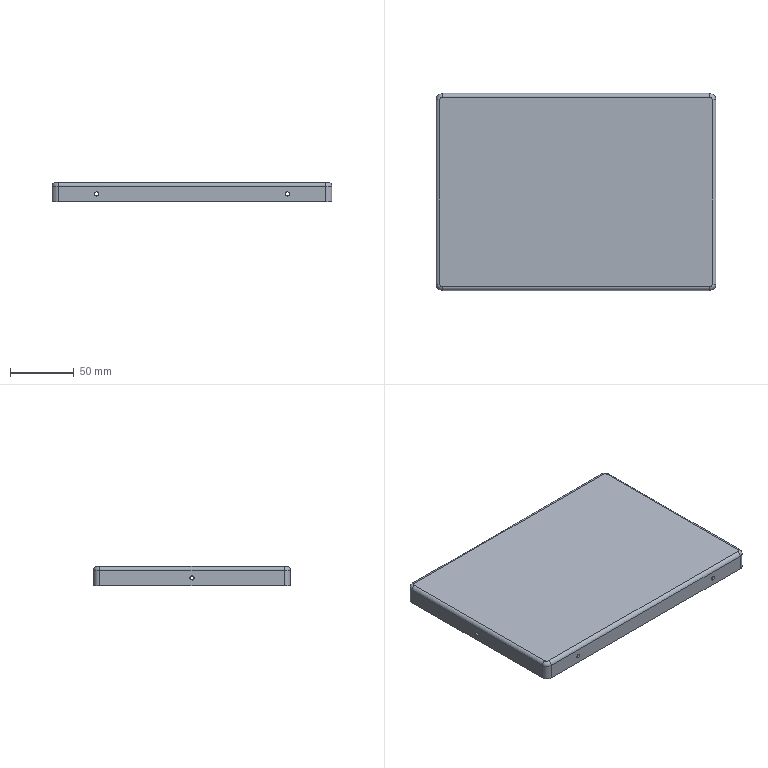Part | NX | features BREP 1 | 1 solid | 47 faces | box 220 x 155 x 15 mm | volume 85900 mm3 | cylinder 28 | plane 11 | torus 8 | commonest cylinder face diameters 3.3 x12 6 x8 2 x4 10 x4
STEP:
#1=CARTESIAN_POINT('',(108.,0.,7.65));
#2=VERTEX_POINT('',#1);
#3=CARTESIAN_POINT('',(110.,0.,7.65));
#4=VERTEX_POINT('',#3);
#5=CARTESIAN_POINT('',(110.,0.,7.65));
#6=DIRECTION('',(1.,0.,0.));
#7=VECTOR('',#6,1000.);
#8=LINE('',#5,#7);
#9=EDGE_CURVE('',#2,#4,#8,.T.);
#10=ORIENTED_EDGE('',*,*,#9,.F.);
#11=CARTESIAN_POINT('',(108.,0.,4.35));
#12=VERTEX_POINT('',#11);
#13=CARTESIAN_POINT('',(108.,0.,6.));
#14=DIRECTION('',(-1.,0.,0.));
#15=DIRECTION('',(0.,0.,1.));
#16=AXIS2_PLACEMENT_3D('',#13,#14,#15);
#17=CIRCLE('',#16,1.65);
#18=EDGE_CURVE('',#2,#12,#17,.T.);
#19=ORIENTED_EDGE('',*,*,#18,.T.);
#20=CARTESIAN_POINT('',(110.,0.,4.35));
#21=VERTEX_POINT('',#20);
#22=CARTESIAN_POINT('',(110.,0.,4.35));
#23=DIRECTION('',(1.,0.,0.));
#24=VECTOR('',#23,1000.);
#25=LINE('',#22,#24);
#26=EDGE_CURVE('',#12,#21,#25,.T.);
#27=ORIENTED_EDGE('',*,*,#26,.T.);
#28=CARTESIAN_POINT('',(110.,0.,6.));
#29=DIRECTION('',(1.,0.,0.));
#30=DIRECTION('',(0.,0.,-1.));
#31=AXIS2_PLACEMENT_3D('',#28,#29,#30);
#32=CIRCLE('',#31,1.65);
#33=EDGE_CURVE('',#21,#4,#32,.T.);
#34=ORIENTED_EDGE('',*,*,#33,.T.);
#35=EDGE_LOOP('',(#10,#19,#27,#34));
#36=FACE_BOUND('',#35,.T.);
#37=CARTESIAN_POINT('',(110.,0.,6.));
#38=DIRECTION('',(1.,0.,0.));
#39=DIRECTION('',(0.,0.,-1.));
#40=AXIS2_PLACEMENT_3D('',#37,#38,#39);
#41=CYLINDRICAL_SURFACE('',#40,1.65);
#42=ADVANCED_FACE('',(#36),#41,.F.);
#43=CARTESIAN_POINT('',(-110.,0.,7.65));
#44=VERTEX_POINT('',#43);
#45=CARTESIAN_POINT('',(-108.,0.,7.65));
#46=VERTEX_POINT('',#45);
#47=CARTESIAN_POINT('',(110.,0.,7.65));
#48=DIRECTION('',(1.,0.,0.));
#49=VECTOR('',#48,1000.);
#50=LINE('',#47,#49);
#51=EDGE_CURVE('',#44,#46,#50,.T.);
#52=ORIENTED_EDGE('',*,*,#51,.F.);
#53=CARTESIAN_POINT('',(-110.,0.,4.35));
#54=VERTEX_POINT('',#53);
#55=CARTESIAN_POINT('',(-110.,0.,6.));
#56=DIRECTION('',(1.,0.,0.));
#57=DIRECTION('',(0.,0.,-1.));
#58=AXIS2_PLACEMENT_3D('',#55,#56,#57);
#59=CIRCLE('',#58,1.65);
#60=EDGE_CURVE('',#54,#44,#59,.T.);
#61=ORIENTED_EDGE('',*,*,#60,.F.);
#62=CARTESIAN_POINT('',(-108.,0.,4.35));
#63=VERTEX_POINT('',#62);
#64=CARTESIAN_POINT('',(110.,0.,4.35));
#65=DIRECTION('',(1.,0.,0.));
#66=VECTOR('',#65,1000.);
#67=LINE('',#64,#66);
#68=EDGE_CURVE('',#54,#63,#67,.T.);
#69=ORIENTED_EDGE('',*,*,#68,.T.);
#70=CARTESIAN_POINT('',(-108.,0.,6.));
#71=DIRECTION('',(1.,0.,0.));
#72=DIRECTION('',(0.,0.,-1.));
#73=AXIS2_PLACEMENT_3D('',#70,#71,#72);
#74=CIRCLE('',#73,1.65);
#75=EDGE_CURVE('',#63,#46,#74,.T.);
#76=ORIENTED_EDGE('',*,*,#75,.T.);
#77=EDGE_LOOP('',(#52,#61,#69,#76));
#78=FACE_BOUND('',#77,.T.);
#79=CARTESIAN_POINT('',(110.,0.,6.));
#80=DIRECTION('',(1.,0.,0.));
#81=DIRECTION('',(0.,0.,-1.));
#82=AXIS2_PLACEMENT_3D('',#79,#80,#81);
#83=CYLINDRICAL_SURFACE('',#82,1.65);
#84=ADVANCED_FACE('',(#78),#83,.F.);
#85=CARTESIAN_POINT('',(-75.,77.5,7.65));
#86=VERTEX_POINT('',#85);
#87=CARTESIAN_POINT('',(-75.,75.5,7.65));
#88=VERTEX_POINT('',#87);
#89=CARTESIAN_POINT('',(-75.,-77.5,7.65));
#90=DIRECTION('',(0.,-1.,0.));
#91=VECTOR('',#90,1000.);
#92=LINE('',#89,#91);
#93=EDGE_CURVE('',#86,#88,#92,.T.);
#94=ORIENTED_EDGE('',*,*,#93,.F.);
#95=CARTESIAN_POINT('',(-75.,77.5,4.35));
#96=VERTEX_POINT('',#95);
#97=CARTESIAN_POINT('',(-75.,77.5,6.));
#98=DIRECTION('',(0.,-1.,0.));
#99=DIRECTION('',(0.,0.,-1.));
#100=AXIS2_PLACEMENT_3D('',#97,#98,#99);
#101=CIRCLE('',#100,1.65);
#102=EDGE_CURVE('',#96,#86,#101,.T.);
#103=ORIENTED_EDGE('',*,*,#102,.F.);
#104=CARTESIAN_POINT('',(-75.,75.5,4.35));
#105=VERTEX_POINT('',#104);
#106=CARTESIAN_POINT('',(-75.,-77.5,4.35));
#107=DIRECTION('',(0.,-1.,0.));
#108=VECTOR('',#107,1000.);
#109=LINE('',#106,#108);
#110=EDGE_CURVE('',#96,#105,#109,.T.);
#111=ORIENTED_EDGE('',*,*,#110,.T.);
#112=CARTESIAN_POINT('',(-75.,75.5,6.));
#113=DIRECTION('',(0.,-1.,0.));
#114=DIRECTION('',(0.,0.,-1.));
#115=AXIS2_PLACEMENT_3D('',#112,#113,#114);
#116=CIRCLE('',#115,1.65);
#117=EDGE_CURVE('',#105,#88,#116,.T.);
#118=ORIENTED_EDGE('',*,*,#117,.T.);
#119=EDGE_LOOP('',(#94,#103,#111,#118));
#120=FACE_BOUND('',#119,.T.);
#121=CARTESIAN_POINT('',(-75.,-77.5,6.));
#122=DIRECTION('',(0.,-1.,0.));
#123=DIRECTION('',(0.,0.,-1.));
#124=AXIS2_PLACEMENT_3D('',#121,#122,#123);
#125=CYLINDRICAL_SURFACE('',#124,1.65);
#126=ADVANCED_FACE('',(#120),#125,.F.);
#127=CARTESIAN_POINT('',(-75.,-75.5,7.65));
#128=VERTEX_POINT('',#127);
#129=CARTESIAN_POINT('',(-75.,-77.5,7.65));
#130=VERTEX_POINT('',#129);
#131=CARTESIAN_POINT('',(-75.,-77.5,7.65));
#132=DIRECTION('',(0.,-1.,0.));
#133=VECTOR('',#132,1000.);
#134=LINE('',#131,#133);
#135=EDGE_CURVE('',#128,#130,#134,.T.);
#136=ORIENTED_EDGE('',*,*,#135,.F.);
#137=CARTESIAN_POINT('',(-75.,-75.5,4.35));
#138=VERTEX_POINT('',#137);
#139=CARTESIAN_POINT('',(-75.,-75.5,6.));
#140=DIRECTION('',(0.,1.,0.));
#141=DIRECTION('',(0.,0.,1.));
#142=AXIS2_PLACEMENT_3D('',#139,#140,#141);
#143=CIRCLE('',#142,1.65);
#144=EDGE_CURVE('',#128,#138,#143,.T.);
#145=ORIENTED_EDGE('',*,*,#144,.T.);
#146=CARTESIAN_POINT('',(-75.,-77.5,4.35));
#147=VERTEX_POINT('',#146);
#148=CARTESIAN_POINT('',(-75.,-77.5,4.35));
#149=DIRECTION('',(0.,-1.,0.));
#150=VECTOR('',#149,1000.);
#151=LINE('',#148,#150);
#152=EDGE_CURVE('',#138,#147,#151,.T.);
#153=ORIENTED_EDGE('',*,*,#152,.T.);
#154=CARTESIAN_POINT('',(-75.,-77.5,6.));
#155=DIRECTION('',(0.,-1.,0.));
#156=DIRECTION('',(0.,0.,-1.));
#157=AXIS2_PLACEMENT_3D('',#154,#155,#156);
#158=CIRCLE('',#157,1.65);
#159=EDGE_CURVE('',#147,#130,#158,.T.);
#160=ORIENTED_EDGE('',*,*,#159,.T.);
#161=EDGE_LOOP('',(#136,#145,#153,#160));
#162=FACE_BOUND('',#161,.T.);
#163=CARTESIAN_POINT('',(-75.,-77.5,6.));
#164=DIRECTION('',(0.,-1.,0.));
#165=DIRECTION('',(0.,0.,-1.));
#166=AXIS2_PLACEMENT_3D('',#163,#164,#165);
#167=CYLINDRICAL_SURFACE('',#166,1.65);
#168=ADVANCED_FACE('',(#162),#167,.F.);
#169=CARTESIAN_POINT('',(75.,-75.5,7.65));
#170=VERTEX_POINT('',#169);
#171=CARTESIAN_POINT('',(75.,-77.5,7.65));
#172=VERTEX_POINT('',#171);
#173=CARTESIAN_POINT('',(75.,-77.5,7.65));
#174=DIRECTION('',(0.,-1.,0.));
#175=VECTOR('',#174,1000.);
#176=LINE('',#173,#175);
#177=EDGE_CURVE('',#170,#172,#176,.T.);
#178=ORIENTED_EDGE('',*,*,#177,.F.);
#179=CARTESIAN_POINT('',(75.,-75.5,4.35));
#180=VERTEX_POINT('',#179);
#181=CARTESIAN_POINT('',(75.,-75.5,6.));
#182=DIRECTION('',(0.,1.,0.));
#183=DIRECTION('',(0.,0.,1.));
#184=AXIS2_PLACEMENT_3D('',#181,#182,#183);
#185=CIRCLE('',#184,1.65);
#186=EDGE_CURVE('',#170,#180,#185,.T.);
#187=ORIENTED_EDGE('',*,*,#186,.T.);
#188=CARTESIAN_POINT('',(75.,-77.5,4.35));
#189=VERTEX_POINT('',#188);
#190=CARTESIAN_POINT('',(75.,-77.5,4.35));
#191=DIRECTION('',(0.,-1.,0.));
#192=VECTOR('',#191,1000.);
#193=LINE('',#190,#192);
#194=EDGE_CURVE('',#180,#189,#193,.T.);
#195=ORIENTED_EDGE('',*,*,#194,.T.);
#196=CARTESIAN_POINT('',(75.,-77.5,6.));
#197=DIRECTION('',(0.,-1.,0.));
#198=DIRECTION('',(0.,0.,-1.));
#199=AXIS2_PLACEMENT_3D('',#196,#197,#198);
#200=CIRCLE('',#199,1.65);
#201=EDGE_CURVE('',#189,#172,#200,.T.);
#202=ORIENTED_EDGE('',*,*,#201,.T.);
#203=EDGE_LOOP('',(#178,#187,#195,#202));
#204=FACE_BOUND('',#203,.T.);
#205=CARTESIAN_POINT('',(75.,-77.5,6.));
#206=DIRECTION('',(0.,-1.,0.));
#207=DIRECTION('',(0.,0.,-1.));
#208=AXIS2_PLACEMENT_3D('',#205,#206,#207);
#209=CYLINDRICAL_SURFACE('',#208,1.65);
#210=ADVANCED_FACE('',(#204),#209,.F.);
#211=CARTESIAN_POINT('',(75.,77.5,7.65));
#212=VERTEX_POINT('',#211);
#213=CARTESIAN_POINT('',(75.,75.5,7.65));
#214=VERTEX_POINT('',#213);
#215=CARTESIAN_POINT('',(75.,-77.5,7.65));
#216=DIRECTION('',(0.,-1.,0.));
#217=VECTOR('',#216,1000.);
#218=LINE('',#215,#217);
#219=EDGE_CURVE('',#212,#214,#218,.T.);
#220=ORIENTED_EDGE('',*,*,#219,.F.);
#221=CARTESIAN_POINT('',(75.,77.5,4.35));
#222=VERTEX_POINT('',#221);
#223=CARTESIAN_POINT('',(75.,77.5,6.));
#224=DIRECTION('',(0.,-1.,0.));
#225=DIRECTION('',(0.,0.,-1.));
#226=AXIS2_PLACEMENT_3D('',#223,#224,#225);
#227=CIRCLE('',#226,1.65);
#228=EDGE_CURVE('',#222,#212,#227,.T.);
#229=ORIENTED_EDGE('',*,*,#228,.F.);
#230=CARTESIAN_POINT('',(75.,75.5,4.35));
#231=VERTEX_POINT('',#230);
#232=CARTESIAN_POINT('',(75.,-77.5,4.35));
#233=DIRECTION('',(0.,-1.,0.));
#234=VECTOR('',#233,1000.);
#235=LINE('',#232,#234);
#236=EDGE_CURVE('',#222,#231,#235,.T.);
#237=ORIENTED_EDGE('',*,*,#236,.T.);
#238=CARTESIAN_POINT('',(75.,75.5,6.));
#239=DIRECTION('',(0.,-1.,0.));
#240=DIRECTION('',(0.,0.,-1.));
#241=AXIS2_PLACEMENT_3D('',#238,#239,#240);
#242=CIRCLE('',#241,1.65);
#243=EDGE_CURVE('',#231,#214,#242,.T.);
#244=ORIENTED_EDGE('',*,*,#243,.T.);
#245=EDGE_LOOP('',(#220,#229,#237,#244));
#246=FACE_BOUND('',#245,.T.);
#247=CARTESIAN_POINT('',(75.,-77.5,6.));
#248=DIRECTION('',(0.,-1.,0.));
#249=DIRECTION('',(0.,0.,-1.));
#250=AXIS2_PLACEMENT_3D('',#247,#248,#249);
#251=CYLINDRICAL_SURFACE('',#250,1.65);
#252=ADVANCED_FACE('',(#246),#251,.F.);
#253=CARTESIAN_POINT('',(-107.,-72.5,13.));
#254=VERTEX_POINT('',#253);
#255=CARTESIAN_POINT('',(-108.,-72.5,12.));
#256=VERTEX_POINT('',#255);
#257=CARTESIAN_POINT('',(-107.,-72.5,12.));
#258=DIRECTION('',(0.,-1.,0.));
#259=DIRECTION('',(-1.,0.,0.));
#260=AXIS2_PLACEMENT_3D('',#257,#258,#259);
#261=CIRCLE('',#260,1.);
#262=EDGE_CURVE('',#254,#256,#261,.T.);
#263=ORIENTED_EDGE('',*,*,#262,.F.);
#264=CARTESIAN_POINT('',(-105.,-74.5,13.));
#265=VERTEX_POINT('',#264);
#266=CARTESIAN_POINT('',(-105.,-72.5,13.));
#267=DIRECTION('',(0.,0.,1.));
#268=DIRECTION('',(1.,0.,0.));
#269=AXIS2_PLACEMENT_3D('',#266,#267,#268);
#270=CIRCLE('',#269,2.);
#271=EDGE_CURVE('',#254,#265,#270,.T.);
#272=ORIENTED_EDGE('',*,*,#271,.T.);
#273=CARTESIAN_POINT('',(-105.,-75.5,12.));
#274=VERTEX_POINT('',#273);
#275=CARTESIAN_POINT('',(-105.,-74.5,12.));
#276=DIRECTION('',(-1.,0.,0.));
#277=DIRECTION('',(0.,-1.,0.));
#278=AXIS2_PLACEMENT_3D('',#275,#276,#277);
#279=CIRCLE('',#278,1.);
#280=EDGE_CURVE('',#274,#265,#279,.T.);
#281=ORIENTED_EDGE('',*,*,#280,.F.);
#282=CARTESIAN_POINT('',(-105.,-72.5,12.));
#283=DIRECTION('',(0.,0.,-1.));
#284=DIRECTION('',(-1.,0.,0.));
#285=AXIS2_PLACEMENT_3D('',#282,#283,#284);
#286=CIRCLE('',#285,3.);
#287=EDGE_CURVE('',#274,#256,#286,.T.);
#288=ORIENTED_EDGE('',*,*,#287,.T.);
#289=EDGE_LOOP('',(#263,#272,#281,#288));
#290=FACE_BOUND('',#289,.T.);
#291=CARTESIAN_POINT('',(-105.,-72.5,12.));
#292=DIRECTION('',(0.,0.,1.));
#293=DIRECTION('',(1.,0.,0.));
#294=AXIS2_PLACEMENT_3D('',#291,#292,#293);
#295=TOROIDAL_SURFACE('',#294,2.,1.);
#296=ADVANCED_FACE('',(#290),#295,.F.);
#297=CARTESIAN_POINT('',(105.,-75.5,12.));
#298=VERTEX_POINT('',#297);
#299=CARTESIAN_POINT('',(105.,-74.5,13.));
#300=VERTEX_POINT('',#299);
#301=CARTESIAN_POINT('',(105.,-74.5,12.));
#302=DIRECTION('',(-1.,0.,0.));
#303=DIRECTION('',(0.,0.,1.));
#304=AXIS2_PLACEMENT_3D('',#301,#302,#303);
#305=CIRCLE('',#304,1.);
#306=EDGE_CURVE('',#298,#300,#305,.T.);
#307=ORIENTED_EDGE('',*,*,#306,.F.);
#308=CARTESIAN_POINT('',(-105.,-75.5,12.));
#309=DIRECTION('',(-1.,0.,0.));
#310=VECTOR('',#309,1000.);
#311=LINE('',#308,#310);
#312=EDGE_CURVE('',#298,#274,#311,.T.);
#313=ORIENTED_EDGE('',*,*,#312,.T.);
#314=ORIENTED_EDGE('',*,*,#280,.T.);
#315=CARTESIAN_POINT('',(105.,-74.5,13.));
#316=DIRECTION('',(1.,0.,0.));
#317=VECTOR('',#316,1000.);
#318=LINE('',#315,#317);
#319=EDGE_CURVE('',#265,#300,#318,.T.);
#320=ORIENTED_EDGE('',*,*,#319,.T.);
#321=EDGE_LOOP('',(#307,#313,#314,#320));
#322=FACE_BOUND('',#321,.T.);
#323=CARTESIAN_POINT('',(105.,-74.5,12.));
#324=DIRECTION('',(-1.,0.,0.));
#325=DIRECTION('',(0.,0.,1.));
#326=AXIS2_PLACEMENT_3D('',#323,#324,#325);
#327=CYLINDRICAL_SURFACE('',#326,1.);
#328=ADVANCED_FACE('',(#322),#327,.F.);
#329=CARTESIAN_POINT('',(-107.,72.5,13.));
#330=VERTEX_POINT('',#329);
#331=CARTESIAN_POINT('',(-108.,72.5,12.));
#332=VERTEX_POINT('',#331);
#333=CARTESIAN_POINT('',(-107.,72.5,12.));
#334=DIRECTION('',(0.,-1.,0.));
#335=DIRECTION('',(0.,0.,1.));
#336=AXIS2_PLACEMENT_3D('',#333,#334,#335);
#337=CIRCLE('',#336,1.);
#338=EDGE_CURVE('',#330,#332,#337,.T.);
#339=ORIENTED_EDGE('',*,*,#338,.F.);
#340=CARTESIAN_POINT('',(-107.,72.5,13.));
#341=DIRECTION('',(0.,-1.,0.));
#342=VECTOR('',#341,1000.);
#343=LINE('',#340,#342);
#344=EDGE_CURVE('',#330,#254,#343,.T.);
#345=ORIENTED_EDGE('',*,*,#344,.T.);
#346=ORIENTED_EDGE('',*,*,#262,.T.);
#347=CARTESIAN_POINT('',(-108.,-72.5,12.));
#348=DIRECTION('',(0.,1.,0.));
#349=VECTOR('',#348,1000.);
#350=LINE('',#347,#349);
#351=EDGE_CURVE('',#256,#332,#350,.T.);
#352=ORIENTED_EDGE('',*,*,#351,.T.);
#353=EDGE_LOOP('',(#339,#345,#346,#352));
#354=FACE_BOUND('',#353,.T.);
#355=CARTESIAN_POINT('',(-107.,72.5,12.));
#356=DIRECTION('',(0.,1.,0.));
#357=DIRECTION('',(0.,0.,1.));
#358=AXIS2_PLACEMENT_3D('',#355,#356,#357);
#359=CYLINDRICAL_SURFACE('',#358,1.);
#360=ADVANCED_FACE('',(#354),#359,.F.);
#361=CARTESIAN_POINT('',(108.,-72.5,12.));
#362=VERTEX_POINT('',#361);
#363=CARTESIAN_POINT('',(107.,-72.5,13.));
#364=VERTEX_POINT('',#363);
#365=CARTESIAN_POINT('',(107.,-72.5,12.));
#366=DIRECTION('',(0.,-1.,0.));
#367=DIRECTION('',(0.,0.,-1.));
#368=AXIS2_PLACEMENT_3D('',#365,#366,#367);
#369=CIRCLE('',#368,1.);
#370=EDGE_CURVE('',#362,#364,#369,.T.);
#371=ORIENTED_EDGE('',*,*,#370,.F.);
#372=CARTESIAN_POINT('',(105.,-72.5,12.));
#373=DIRECTION('',(0.,0.,-1.));
#374=DIRECTION('',(-1.,0.,0.));
#375=AXIS2_PLACEMENT_3D('',#372,#373,#374);
#376=CIRCLE('',#375,3.);
#377=EDGE_CURVE('',#362,#298,#376,.T.);
#378=ORIENTED_EDGE('',*,*,#377,.T.);
#379=ORIENTED_EDGE('',*,*,#306,.T.);
#380=CARTESIAN_POINT('',(105.,-72.5,13.));
#381=DIRECTION('',(0.,0.,1.));
#382=DIRECTION('',(1.,0.,0.));
#383=AXIS2_PLACEMENT_3D('',#380,#381,#382);
#384=CIRCLE('',#383,2.);
#385=EDGE_CURVE('',#300,#364,#384,.T.);
#386=ORIENTED_EDGE('',*,*,#385,.T.);
#387=EDGE_LOOP('',(#371,#378,#379,#386));
#388=FACE_BOUND('',#387,.T.);
#389=CARTESIAN_POINT('',(105.,-72.5,12.));
#390=DIRECTION('',(0.,0.,1.));
#391=DIRECTION('',(1.,0.,0.));
#392=AXIS2_PLACEMENT_3D('',#389,#390,#391);
#393=TOROIDAL_SURFACE('',#392,2.,1.);
#394=ADVANCED_FACE('',(#388),#393,.F.);
#395=CARTESIAN_POINT('',(-105.,74.5,13.));
#396=VERTEX_POINT('',#395);
#397=CARTESIAN_POINT('',(-105.,75.5,12.));
#398=VERTEX_POINT('',#397);
#399=CARTESIAN_POINT('',(-105.,74.5,12.));
#400=DIRECTION('',(-1.,0.,0.));
#401=DIRECTION('',(0.,1.,0.));
#402=AXIS2_PLACEMENT_3D('',#399,#400,#401);
#403=CIRCLE('',#402,1.);
#404=EDGE_CURVE('',#396,#398,#403,.T.);
#405=ORIENTED_EDGE('',*,*,#404,.F.);
#406=CARTESIAN_POINT('',(-105.,72.5,13.));
#407=DIRECTION('',(0.,0.,1.));
#408=DIRECTION('',(1.,0.,0.));
#409=AXIS2_PLACEMENT_3D('',#406,#407,#408);
#410=CIRCLE('',#409,2.);
#411=EDGE_CURVE('',#396,#330,#410,.T.);
#412=ORIENTED_EDGE('',*,*,#411,.T.);
#413=ORIENTED_EDGE('',*,*,#338,.T.);
#414=CARTESIAN_POINT('',(-105.,72.5,12.));
#415=DIRECTION('',(0.,0.,-1.));
#416=DIRECTION('',(-1.,0.,0.));
#417=AXIS2_PLACEMENT_3D('',#414,#415,#416);
#418=CIRCLE('',#417,3.);
#419=EDGE_CURVE('',#332,#398,#418,.T.);
#420=ORIENTED_EDGE('',*,*,#419,.T.);
#421=EDGE_LOOP('',(#405,#412,#413,#420));
#422=FACE_BOUND('',#421,.T.);
#423=CARTESIAN_POINT('',(-105.,72.5,12.));
#424=DIRECTION('',(0.,0.,1.));
#425=DIRECTION('',(1.,0.,0.));
#426=AXIS2_PLACEMENT_3D('',#423,#424,#425);
#427=TOROIDAL_SURFACE('',#426,2.,1.);
#428=ADVANCED_FACE('',(#422),#427,.F.);
#429=CARTESIAN_POINT('',(108.,72.5,12.));
#430=VERTEX_POINT('',#429);
#431=CARTESIAN_POINT('',(107.,72.5,13.));
#432=VERTEX_POINT('',#431);
#433=CARTESIAN_POINT('',(107.,72.5,12.));
#434=DIRECTION('',(0.,-1.,0.));
#435=DIRECTION('',(0.,0.,-1.));
#436=AXIS2_PLACEMENT_3D('',#433,#434,#435);
#437=CIRCLE('',#436,1.);
#438=EDGE_CURVE('',#430,#432,#437,.T.);
#439=ORIENTED_EDGE('',*,*,#438,.F.);
#440=CARTESIAN_POINT('',(108.,-72.5,12.));
#441=DIRECTION('',(0.,-1.,0.));
#442=VECTOR('',#441,1000.);
#443=LINE('',#440,#442);
#444=EDGE_CURVE('',#430,#362,#443,.T.);
#445=ORIENTED_EDGE('',*,*,#444,.T.);
#446=ORIENTED_EDGE('',*,*,#370,.T.);
#447=CARTESIAN_POINT('',(107.,72.5,13.));
#448=DIRECTION('',(0.,1.,0.));
#449=VECTOR('',#448,1000.);
#450=LINE('',#447,#449);
#451=EDGE_CURVE('',#364,#432,#450,.T.);
#452=ORIENTED_EDGE('',*,*,#451,.T.);
#453=EDGE_LOOP('',(#439,#445,#446,#452));
#454=FACE_BOUND('',#453,.T.);
#455=CARTESIAN_POINT('',(107.,72.5,12.));
#456=DIRECTION('',(0.,-1.,0.));
#457=DIRECTION('',(0.,0.,-1.));
#458=AXIS2_PLACEMENT_3D('',#455,#456,#457);
#459=CYLINDRICAL_SURFACE('',#458,1.);
#460=ADVANCED_FACE('',(#454),#459,.F.);
#461=CARTESIAN_POINT('',(105.,74.5,13.));
#462=VERTEX_POINT('',#461);
#463=CARTESIAN_POINT('',(105.,75.5,12.));
#464=VERTEX_POINT('',#463);
#465=CARTESIAN_POINT('',(105.,74.5,12.));
#466=DIRECTION('',(-1.,0.,0.));
#467=DIRECTION('',(0.,0.,-1.));
#468=AXIS2_PLACEMENT_3D('',#465,#466,#467);
#469=CIRCLE('',#468,1.);
#470=EDGE_CURVE('',#462,#464,#469,.T.);
#471=ORIENTED_EDGE('',*,*,#470,.F.);
#472=CARTESIAN_POINT('',(105.,74.5,13.));
#473=DIRECTION('',(-1.,0.,0.));
#474=VECTOR('',#473,1000.);
#475=LINE('',#472,#474);
#476=EDGE_CURVE('',#462,#396,#475,.T.);
#477=ORIENTED_EDGE('',*,*,#476,.T.);
#478=ORIENTED_EDGE('',*,*,#404,.T.);
#479=CARTESIAN_POINT('',(-105.,75.5,12.));
#480=DIRECTION('',(1.,0.,0.));
#481=VECTOR('',#480,1000.);
#482=LINE('',#479,#481);
#483=EDGE_CURVE('',#398,#464,#482,.T.);
#484=ORIENTED_EDGE('',*,*,#483,.T.);
#485=EDGE_LOOP('',(#471,#477,#478,#484));
#486=FACE_BOUND('',#485,.T.);
#487=CARTESIAN_POINT('',(105.,74.5,12.));
#488=DIRECTION('',(1.,0.,0.));
#489=DIRECTION('',(0.,0.,-1.));
#490=AXIS2_PLACEMENT_3D('',#487,#488,#489);
#491=CYLINDRICAL_SURFACE('',#490,1.);
#492=ADVANCED_FACE('',(#486),#491,.F.);
#493=ORIENTED_EDGE('',*,*,#438,.T.);
#494=CARTESIAN_POINT('',(105.,72.5,13.));
#495=DIRECTION('',(0.,0.,1.));
#496=DIRECTION('',(1.,0.,0.));
#497=AXIS2_PLACEMENT_3D('',#494,#495,#496);
#498=CIRCLE('',#497,2.);
#499=EDGE_CURVE('',#432,#462,#498,.T.);
#500=ORIENTED_EDGE('',*,*,#499,.T.);
#501=ORIENTED_EDGE('',*,*,#470,.T.);
#502=CARTESIAN_POINT('',(105.,72.5,12.));
#503=DIRECTION('',(0.,0.,-1.));
#504=DIRECTION('',(-1.,0.,0.));
#505=AXIS2_PLACEMENT_3D('',#502,#503,#504);
#506=CIRCLE('',#505,3.);
#507=EDGE_CURVE('',#464,#430,#506,.T.);
#508=ORIENTED_EDGE('',*,*,#507,.T.);
#509=EDGE_LOOP('',(#493,#500,#501,#508));
#510=FACE_BOUND('',#509,.T.);
#511=CARTESIAN_POINT('',(105.,72.5,12.));
#512=DIRECTION('',(0.,0.,1.));
#513=DIRECTION('',(1.,0.,0.));
#514=AXIS2_PLACEMENT_3D('',#511,#512,#513);
#515=TOROIDAL_SURFACE('',#514,2.,1.);
#516=ADVANCED_FACE('',(#510),#515,.F.);
#517=ORIENTED_EDGE('',*,*,#344,.F.);
#518=ORIENTED_EDGE('',*,*,#411,.F.);
#519=ORIENTED_EDGE('',*,*,#476,.F.);
#520=ORIENTED_EDGE('',*,*,#499,.F.);
#521=ORIENTED_EDGE('',*,*,#451,.F.);
#522=ORIENTED_EDGE('',*,*,#385,.F.);
#523=ORIENTED_EDGE('',*,*,#319,.F.);
#524=ORIENTED_EDGE('',*,*,#271,.F.);
#525=EDGE_LOOP('',(#517,#518,#519,#520,#521,#522,#523,#524));
#526=FACE_BOUND('',#525,.T.);
#527=CARTESIAN_POINT('',(105.,72.5,13.));
#528=DIRECTION('',(0.,0.,1.));
#529=DIRECTION('',(1.,0.,0.));
#530=AXIS2_PLACEMENT_3D('',#527,#528,#529);
#531=PLANE('',#530);
#532=ADVANCED_FACE('',(#526),#531,.F.);
#533=CARTESIAN_POINT('',(108.,72.5,0.));
#534=VERTEX_POINT('',#533);
#535=CARTESIAN_POINT('',(108.,72.5,15.));
#536=DIRECTION('',(0.,0.,-1.));
#537=VECTOR('',#536,1000.);
#538=LINE('',#535,#537);
#539=EDGE_CURVE('',#430,#534,#538,.T.);
#540=ORIENTED_EDGE('',*,*,#539,.T.);
#541=CARTESIAN_POINT('',(108.,-72.5,0.));
#542=VERTEX_POINT('',#541);
#543=CARTESIAN_POINT('',(108.,-72.5,0.));
#544=DIRECTION('',(0.,1.,0.));
#545=VECTOR('',#544,1000.);
#546=LINE('',#543,#545);
#547=EDGE_CURVE('',#542,#534,#546,.T.);
#548=ORIENTED_EDGE('',*,*,#547,.F.);
#549=CARTESIAN_POINT('',(108.,-72.5,15.));
#550=DIRECTION('',(0.,0.,-1.));
#551=VECTOR('',#550,1000.);
#552=LINE('',#549,#551);
#553=EDGE_CURVE('',#362,#542,#552,.T.);
#554=ORIENTED_EDGE('',*,*,#553,.F.);
#555=ORIENTED_EDGE('',*,*,#444,.F.);
#556=EDGE_LOOP('',(#540,#548,#554,#555));
#557=FACE_BOUND('',#556,.T.);
#558=CARTESIAN_POINT('',(108.,0.,6.));
#559=DIRECTION('',(-1.,0.,0.));
#560=DIRECTION('',(0.,0.,1.));
#561=AXIS2_PLACEMENT_3D('',#558,#559,#560);
#562=CIRCLE('',#561,1.65);
#563=EDGE_CURVE('',#12,#2,#562,.T.);
#564=ORIENTED_EDGE('',*,*,#563,.F.);
#565=ORIENTED_EDGE('',*,*,#18,.F.);
#566=EDGE_LOOP('',(#564,#565));
#567=FACE_BOUND('',#566,.T.);
#568=CARTESIAN_POINT('',(108.,-72.5,15.));
#569=DIRECTION('',(-1.,0.,0.));
#570=DIRECTION('',(0.,0.,1.));
#571=AXIS2_PLACEMENT_3D('',#568,#569,#570);
#572=PLANE('',#571);
#573=ADVANCED_FACE('',(#557,#567),#572,.T.);
#574=ORIENTED_EDGE('',*,*,#553,.T.);
#575=CARTESIAN_POINT('',(105.,-75.5,0.));
#576=VERTEX_POINT('',#575);
#577=CARTESIAN_POINT('',(105.,-72.5,0.));
#578=DIRECTION('',(0.,0.,1.));
#579=DIRECTION('',(1.,0.,0.));
#580=AXIS2_PLACEMENT_3D('',#577,#578,#579);
#581=CIRCLE('',#580,3.);
#582=EDGE_CURVE('',#576,#542,#581,.T.);
#583=ORIENTED_EDGE('',*,*,#582,.F.);
#584=CARTESIAN_POINT('',(105.,-75.5,15.));
#585=DIRECTION('',(0.,0.,-1.));
#586=VECTOR('',#585,1000.);
#587=LINE('',#584,#586);
#588=EDGE_CURVE('',#298,#576,#587,.T.);
#589=ORIENTED_EDGE('',*,*,#588,.F.);
#590=ORIENTED_EDGE('',*,*,#377,.F.);
#591=EDGE_LOOP('',(#574,#583,#589,#590));
#592=FACE_BOUND('',#591,.T.);
#593=CARTESIAN_POINT('',(105.,-72.5,15.));
#594=DIRECTION('',(0.,0.,-1.));
#595=DIRECTION('',(-1.,0.,0.));
#596=AXIS2_PLACEMENT_3D('',#593,#594,#595);
#597=CYLINDRICAL_SURFACE('',#596,3.);
#598=ADVANCED_FACE('',(#592),#597,.F.);
#599=ORIENTED_EDGE('',*,*,#588,.T.);
#600=CARTESIAN_POINT('',(-105.,-75.5,0.));
#601=VERTEX_POINT('',#600);
#602=CARTESIAN_POINT('',(-105.,-75.5,0.));
#603=DIRECTION('',(1.,0.,0.));
#604=VECTOR('',#603,1000.);
#605=LINE('',#602,#604);
#606=EDGE_CURVE('',#601,#576,#605,.T.);
#607=ORIENTED_EDGE('',*,*,#606,.F.);
#608=CARTESIAN_POINT('',(-105.,-75.5,15.));
#609=DIRECTION('',(0.,0.,-1.));
#610=VECTOR('',#609,1000.);
#611=LINE('',#608,#610);
#612=EDGE_CURVE('',#274,#601,#611,.T.);
#613=ORIENTED_EDGE('',*,*,#612,.F.);
#614=ORIENTED_EDGE('',*,*,#312,.F.);
#615=EDGE_LOOP('',(#599,#607,#613,#614));
#616=FACE_BOUND('',#615,.T.);
#617=CARTESIAN_POINT('',(75.,-75.5,6.));
#618=DIRECTION('',(0.,1.,0.));
#619=DIRECTION('',(0.,0.,1.));
#620=AXIS2_PLACEMENT_3D('',#617,#618,#619);
#621=CIRCLE('',#620,1.65);
#622=EDGE_CURVE('',#180,#170,#621,.T.);
#623=ORIENTED_EDGE('',*,*,#622,.F.);
#624=ORIENTED_EDGE('',*,*,#186,.F.);
#625=EDGE_LOOP('',(#623,#624));
#626=FACE_BOUND('',#625,.T.);
#627=CARTESIAN_POINT('',(-75.,-75.5,6.));
#628=DIRECTION('',(0.,1.,0.));
#629=DIRECTION('',(0.,0.,1.));
#630=AXIS2_PLACEMENT_3D('',#627,#628,#629);
#631=CIRCLE('',#630,1.65);
#632=EDGE_CURVE('',#138,#128,#631,.T.);
#633=ORIENTED_EDGE('',*,*,#632,.F.);
#634=ORIENTED_EDGE('',*,*,#144,.F.);
#635=EDGE_LOOP('',(#633,#634));
#636=FACE_BOUND('',#635,.T.);
#637=CARTESIAN_POINT('',(-105.,-75.5,15.));
#638=DIRECTION('',(0.,1.,0.));
#639=DIRECTION('',(0.,0.,1.));
#640=AXIS2_PLACEMENT_3D('',#637,#638,#639);
#641=PLANE('',#640);
#642=ADVANCED_FACE('',(#616,#626,#636),#641,.T.);
#643=ORIENTED_EDGE('',*,*,#612,.T.);
#644=CARTESIAN_POINT('',(-108.,-72.5,0.));
#645=VERTEX_POINT('',#644);
#646=CARTESIAN_POINT('',(-105.,-72.5,0.));
#647=DIRECTION('',(0.,0.,1.));
#648=DIRECTION('',(1.,0.,0.));
#649=AXIS2_PLACEMENT_3D('',#646,#647,#648);
#650=CIRCLE('',#649,3.);
#651=EDGE_CURVE('',#645,#601,#650,.T.);
#652=ORIENTED_EDGE('',*,*,#651,.F.);
#653=CARTESIAN_POINT('',(-108.,-72.5,15.));
#654=DIRECTION('',(0.,0.,-1.));
#655=VECTOR('',#654,1000.);
#656=LINE('',#653,#655);
#657=EDGE_CURVE('',#256,#645,#656,.T.);
#658=ORIENTED_EDGE('',*,*,#657,.F.);
#659=ORIENTED_EDGE('',*,*,#287,.F.);
#660=EDGE_LOOP('',(#643,#652,#658,#659));
#661=FACE_BOUND('',#660,.T.);
#662=CARTESIAN_POINT('',(-105.,-72.5,15.));
#663=DIRECTION('',(0.,0.,-1.));
#664=DIRECTION('',(-1.,0.,0.));
#665=AXIS2_PLACEMENT_3D('',#662,#663,#664);
#666=CYLINDRICAL_SURFACE('',#665,3.);
#667=ADVANCED_FACE('',(#661),#666,.F.);
#668=ORIENTED_EDGE('',*,*,#657,.T.);
#669=CARTESIAN_POINT('',(-108.,72.5,0.));
#670=VERTEX_POINT('',#669);
#671=CARTESIAN_POINT('',(-108.,-72.5,0.));
#672=DIRECTION('',(0.,-1.,0.));
#673=VECTOR('',#672,1000.);
#674=LINE('',#671,#673);
#675=EDGE_CURVE('',#670,#645,#674,.T.);
#676=ORIENTED_EDGE('',*,*,#675,.F.);
#677=CARTESIAN_POINT('',(-108.,72.5,15.));
#678=DIRECTION('',(0.,0.,-1.));
#679=VECTOR('',#678,1000.);
#680=LINE('',#677,#679);
#681=EDGE_CURVE('',#332,#670,#680,.T.);
#682=ORIENTED_EDGE('',*,*,#681,.F.);
#683=ORIENTED_EDGE('',*,*,#351,.F.);
#684=EDGE_LOOP('',(#668,#676,#682,#683));
#685=FACE_BOUND('',#684,.T.);
#686=ORIENTED_EDGE('',*,*,#75,.F.);
#687=CARTESIAN_POINT('',(-108.,0.,6.));
#688=DIRECTION('',(1.,0.,0.));
#689=DIRECTION('',(0.,0.,-1.));
#690=AXIS2_PLACEMENT_3D('',#687,#688,#689);
#691=CIRCLE('',#690,1.65);
#692=EDGE_CURVE('',#46,#63,#691,.T.);
#693=ORIENTED_EDGE('',*,*,#692,.F.);
#694=EDGE_LOOP('',(#686,#693));
#695=FACE_BOUND('',#694,.T.);
#696=CARTESIAN_POINT('',(-108.,-72.5,15.));
#697=DIRECTION('',(1.,0.,0.));
#698=DIRECTION('',(0.,0.,-1.));
#699=AXIS2_PLACEMENT_3D('',#696,#697,#698);
#700=PLANE('',#699);
#701=ADVANCED_FACE('',(#685,#695),#700,.T.);
#702=ORIENTED_EDGE('',*,*,#681,.T.);
#703=CARTESIAN_POINT('',(-105.,75.5,0.));
#704=VERTEX_POINT('',#703);
#705=CARTESIAN_POINT('',(-105.,72.5,0.));
#706=DIRECTION('',(0.,0.,1.));
#707=DIRECTION('',(1.,0.,0.));
#708=AXIS2_PLACEMENT_3D('',#705,#706,#707);
#709=CIRCLE('',#708,3.);
#710=EDGE_CURVE('',#704,#670,#709,.T.);
#711=ORIENTED_EDGE('',*,*,#710,.F.);
#712=CARTESIAN_POINT('',(-105.,75.5,15.));
#713=DIRECTION('',(0.,0.,-1.));
#714=VECTOR('',#713,1000.);
#715=LINE('',#712,#714);
#716=EDGE_CURVE('',#398,#704,#715,.T.);
#717=ORIENTED_EDGE('',*,*,#716,.F.);
#718=ORIENTED_EDGE('',*,*,#419,.F.);
#719=EDGE_LOOP('',(#702,#711,#717,#718));
#720=FACE_BOUND('',#719,.T.);
#721=CARTESIAN_POINT('',(-105.,72.5,15.));
#722=DIRECTION('',(0.,0.,-1.));
#723=DIRECTION('',(-1.,0.,0.));
#724=AXIS2_PLACEMENT_3D('',#721,#722,#723);
#725=CYLINDRICAL_SURFACE('',#724,3.);
#726=ADVANCED_FACE('',(#720),#725,.F.);
#727=ORIENTED_EDGE('',*,*,#716,.T.);
#728=CARTESIAN_POINT('',(105.,75.5,0.));
#729=VERTEX_POINT('',#728);
#730=CARTESIAN_POINT('',(-105.,75.5,0.));
#731=DIRECTION('',(-1.,0.,0.));
#732=VECTOR('',#731,1000.);
#733=LINE('',#730,#732);
#734=EDGE_CURVE('',#729,#704,#733,.T.);
#735=ORIENTED_EDGE('',*,*,#734,.F.);
#736=CARTESIAN_POINT('',(105.,75.5,15.));
#737=DIRECTION('',(0.,0.,-1.));
#738=VECTOR('',#737,1000.);
#739=LINE('',#736,#738);
#740=EDGE_CURVE('',#464,#729,#739,.T.);
#741=ORIENTED_EDGE('',*,*,#740,.F.);
#742=ORIENTED_EDGE('',*,*,#483,.F.);
#743=EDGE_LOOP('',(#727,#735,#741,#742));
#744=FACE_BOUND('',#743,.T.);
#745=ORIENTED_EDGE('',*,*,#243,.F.);
#746=CARTESIAN_POINT('',(75.,75.5,6.));
#747=DIRECTION('',(0.,-1.,0.));
#748=DIRECTION('',(0.,0.,-1.));
#749=AXIS2_PLACEMENT_3D('',#746,#747,#748);
#750=CIRCLE('',#749,1.65);
#751=EDGE_CURVE('',#214,#231,#750,.T.);
#752=ORIENTED_EDGE('',*,*,#751,.F.);
#753=EDGE_LOOP('',(#745,#752));
#754=FACE_BOUND('',#753,.T.);
#755=ORIENTED_EDGE('',*,*,#117,.F.);
#756=CARTESIAN_POINT('',(-75.,75.5,6.));
#757=DIRECTION('',(0.,-1.,0.));
#758=DIRECTION('',(0.,0.,-1.));
#759=AXIS2_PLACEMENT_3D('',#756,#757,#758);
#760=CIRCLE('',#759,1.65);
#761=EDGE_CURVE('',#88,#105,#760,.T.);
#762=ORIENTED_EDGE('',*,*,#761,.F.);
#763=EDGE_LOOP('',(#755,#762));
#764=FACE_BOUND('',#763,.T.);
#765=CARTESIAN_POINT('',(-105.,75.5,15.));
#766=DIRECTION('',(0.,-1.,0.));
#767=DIRECTION('',(0.,0.,-1.));
#768=AXIS2_PLACEMENT_3D('',#765,#766,#767);
#769=PLANE('',#768);
#770=ADVANCED_FACE('',(#744,#754,#764),#769,.T.);
#771=ORIENTED_EDGE('',*,*,#740,.T.);
#772=CARTESIAN_POINT('',(105.,72.5,0.));
#773=DIRECTION('',(0.,0.,1.));
#774=DIRECTION('',(1.,0.,0.));
#775=AXIS2_PLACEMENT_3D('',#772,#773,#774);
#776=CIRCLE('',#775,3.);
#777=EDGE_CURVE('',#534,#729,#776,.T.);
#778=ORIENTED_EDGE('',*,*,#777,.F.);
#779=ORIENTED_EDGE('',*,*,#539,.F.);
#780=ORIENTED_EDGE('',*,*,#507,.F.);
#781=EDGE_LOOP('',(#771,#778,#779,#780));
#782=FACE_BOUND('',#781,.T.);
#783=CARTESIAN_POINT('',(105.,72.5,15.));
#784=DIRECTION('',(0.,0.,-1.));
#785=DIRECTION('',(-1.,0.,0.));
#786=AXIS2_PLACEMENT_3D('',#783,#784,#785);
#787=CYLINDRICAL_SURFACE('',#786,3.);
#788=ADVANCED_FACE('',(#782),#787,.F.);
#789=CARTESIAN_POINT('',(-107.,-72.5,15.));
#790=VERTEX_POINT('',#789);
#791=CARTESIAN_POINT('',(-110.,-72.5,12.));
#792=VERTEX_POINT('',#791);
#793=CARTESIAN_POINT('',(-107.,-72.5,12.));
#794=DIRECTION('',(0.,-1.,0.));
#795=DIRECTION('',(0.,0.,-1.));
#796=AXIS2_PLACEMENT_3D('',#793,#794,#795);
#797=CIRCLE('',#796,3.);
#798=EDGE_CURVE('',#790,#792,#797,.T.);
#799=ORIENTED_EDGE('',*,*,#798,.T.);
#800=CARTESIAN_POINT('',(-105.,-77.5,12.));
#801=VERTEX_POINT('',#800);
#802=CARTESIAN_POINT('',(-105.,-72.5,12.));
#803=DIRECTION('',(0.,0.,-1.));
#804=DIRECTION('',(1.,0.,0.));
#805=AXIS2_PLACEMENT_3D('',#802,#803,#804);
#806=CIRCLE('',#805,5.);
#807=EDGE_CURVE('',#801,#792,#806,.T.);
#808=ORIENTED_EDGE('',*,*,#807,.F.);
#809=CARTESIAN_POINT('',(-105.,-74.5,15.));
#810=VERTEX_POINT('',#809);
#811=CARTESIAN_POINT('',(-105.,-74.5,12.));
#812=DIRECTION('',(-1.,0.,0.));
#813=DIRECTION('',(0.,0.,1.));
#814=AXIS2_PLACEMENT_3D('',#811,#812,#813);
#815=CIRCLE('',#814,3.);
#816=EDGE_CURVE('',#801,#810,#815,.T.);
#817=ORIENTED_EDGE('',*,*,#816,.T.);
#818=CARTESIAN_POINT('',(-105.,-72.5,15.));
#819=DIRECTION('',(0.,0.,1.));
#820=DIRECTION('',(1.,0.,0.));
#821=AXIS2_PLACEMENT_3D('',#818,#819,#820);
#822=CIRCLE('',#821,2.);
#823=EDGE_CURVE('',#790,#810,#822,.T.);
#824=ORIENTED_EDGE('',*,*,#823,.F.);
#825=EDGE_LOOP('',(#799,#808,#817,#824));
#826=FACE_BOUND('',#825,.T.);
#827=CARTESIAN_POINT('',(-105.,-72.5,12.));
#828=DIRECTION('',(0.,0.,1.));
#829=DIRECTION('',(1.,0.,0.));
#830=AXIS2_PLACEMENT_3D('',#827,#828,#829);
#831=DEGENERATE_TOROIDAL_SURFACE('',#830,2.,3.,.T.);
#832=ADVANCED_FACE('',(#826),#831,.T.);
#833=CARTESIAN_POINT('',(105.,-77.5,12.));
#834=VERTEX_POINT('',#833);
#835=CARTESIAN_POINT('',(105.,-74.5,15.));
#836=VERTEX_POINT('',#835);
#837=CARTESIAN_POINT('',(105.,-74.5,12.));
#838=DIRECTION('',(-1.,0.,0.));
#839=DIRECTION('',(0.,0.,1.));
#840=AXIS2_PLACEMENT_3D('',#837,#838,#839);
#841=CIRCLE('',#840,3.);
#842=EDGE_CURVE('',#834,#836,#841,.T.);
#843=ORIENTED_EDGE('',*,*,#842,.T.);
#844=CARTESIAN_POINT('',(105.,-74.5,15.));
#845=DIRECTION('',(1.,0.,0.));
#846=VECTOR('',#845,1000.);
#847=LINE('',#844,#846);
#848=EDGE_CURVE('',#810,#836,#847,.T.);
#849=ORIENTED_EDGE('',*,*,#848,.F.);
#850=ORIENTED_EDGE('',*,*,#816,.F.);
#851=CARTESIAN_POINT('',(-105.,-77.5,12.));
#852=DIRECTION('',(-1.,0.,0.));
#853=VECTOR('',#852,1000.);
#854=LINE('',#851,#853);
#855=EDGE_CURVE('',#834,#801,#854,.T.);
#856=ORIENTED_EDGE('',*,*,#855,.F.);
#857=EDGE_LOOP('',(#843,#849,#850,#856));
#858=FACE_BOUND('',#857,.T.);
#859=CARTESIAN_POINT('',(105.,-74.5,12.));
#860=DIRECTION('',(-1.,0.,0.));
#861=DIRECTION('',(0.,0.,1.));
#862=AXIS2_PLACEMENT_3D('',#859,#860,#861);
#863=CYLINDRICAL_SURFACE('',#862,3.);
#864=ADVANCED_FACE('',(#858),#863,.T.);
#865=CARTESIAN_POINT('',(-107.,72.5,15.));
#866=VERTEX_POINT('',#865);
#867=CARTESIAN_POINT('',(-110.,72.5,12.));
#868=VERTEX_POINT('',#867);
#869=CARTESIAN_POINT('',(-107.,72.5,12.));
#870=DIRECTION('',(0.,-1.,0.));
#871=DIRECTION('',(0.,0.,-1.));
#872=AXIS2_PLACEMENT_3D('',#869,#870,#871);
#873=CIRCLE('',#872,3.);
#874=EDGE_CURVE('',#866,#868,#873,.T.);
#875=ORIENTED_EDGE('',*,*,#874,.T.);
#876=CARTESIAN_POINT('',(-110.,72.5,12.));
#877=DIRECTION('',(0.,1.,0.));
#878=VECTOR('',#877,1000.);
#879=LINE('',#876,#878);
#880=EDGE_CURVE('',#792,#868,#879,.T.);
#881=ORIENTED_EDGE('',*,*,#880,.F.);
#882=ORIENTED_EDGE('',*,*,#798,.F.);
#883=CARTESIAN_POINT('',(-107.,-72.5,15.));
#884=DIRECTION('',(0.,-1.,0.));
#885=VECTOR('',#884,1000.);
#886=LINE('',#883,#885);
#887=EDGE_CURVE('',#866,#790,#886,.T.);
#888=ORIENTED_EDGE('',*,*,#887,.F.);
#889=EDGE_LOOP('',(#875,#881,#882,#888));
#890=FACE_BOUND('',#889,.T.);
#891=CARTESIAN_POINT('',(-107.,72.5,12.));
#892=DIRECTION('',(0.,1.,0.));
#893=DIRECTION('',(0.,0.,1.));
#894=AXIS2_PLACEMENT_3D('',#891,#892,#893);
#895=CYLINDRICAL_SURFACE('',#894,3.);
#896=ADVANCED_FACE('',(#890),#895,.T.);
#897=CARTESIAN_POINT('',(110.,-72.5,12.));
#898=VERTEX_POINT('',#897);
#899=CARTESIAN_POINT('',(107.,-72.5,15.));
#900=VERTEX_POINT('',#899);
#901=CARTESIAN_POINT('',(107.,-72.5,12.));
#902=DIRECTION('',(0.,-1.,0.));
#903=DIRECTION('',(0.,0.,-1.));
#904=AXIS2_PLACEMENT_3D('',#901,#902,#903);
#905=CIRCLE('',#904,3.);
#906=EDGE_CURVE('',#898,#900,#905,.T.);
#907=ORIENTED_EDGE('',*,*,#906,.T.);
#908=CARTESIAN_POINT('',(105.,-72.5,15.));
#909=DIRECTION('',(0.,0.,1.));
#910=DIRECTION('',(1.,0.,0.));
#911=AXIS2_PLACEMENT_3D('',#908,#909,#910);
#912=CIRCLE('',#911,2.);
#913=EDGE_CURVE('',#836,#900,#912,.T.);
#914=ORIENTED_EDGE('',*,*,#913,.F.);
#915=ORIENTED_EDGE('',*,*,#842,.F.);
#916=CARTESIAN_POINT('',(105.,-72.5,12.));
#917=DIRECTION('',(0.,0.,-1.));
#918=DIRECTION('',(1.,0.,0.));
#919=AXIS2_PLACEMENT_3D('',#916,#917,#918);
#920=CIRCLE('',#919,5.);
#921=EDGE_CURVE('',#898,#834,#920,.T.);
#922=ORIENTED_EDGE('',*,*,#921,.F.);
#923=EDGE_LOOP('',(#907,#914,#915,#922));
#924=FACE_BOUND('',#923,.T.);
#925=CARTESIAN_POINT('',(105.,-72.5,12.));
#926=DIRECTION('',(0.,0.,1.));
#927=DIRECTION('',(1.,0.,0.));
#928=AXIS2_PLACEMENT_3D('',#925,#926,#927);
#929=DEGENERATE_TOROIDAL_SURFACE('',#928,2.,3.,.T.);
#930=ADVANCED_FACE('',(#924),#929,.T.);
#931=CARTESIAN_POINT('',(-105.,74.5,15.));
#932=VERTEX_POINT('',#931);
#933=CARTESIAN_POINT('',(-105.,77.5,12.));
#934=VERTEX_POINT('',#933);
#935=CARTESIAN_POINT('',(-105.,74.5,12.));
#936=DIRECTION('',(-1.,0.,0.));
#937=DIRECTION('',(0.,0.,1.));
#938=AXIS2_PLACEMENT_3D('',#935,#936,#937);
#939=CIRCLE('',#938,3.);
#940=EDGE_CURVE('',#932,#934,#939,.T.);
#941=ORIENTED_EDGE('',*,*,#940,.T.);
#942=CARTESIAN_POINT('',(-105.,72.5,12.));
#943=DIRECTION('',(0.,0.,-1.));
#944=DIRECTION('',(1.,0.,0.));
#945=AXIS2_PLACEMENT_3D('',#942,#943,#944);
#946=CIRCLE('',#945,5.);
#947=EDGE_CURVE('',#868,#934,#946,.T.);
#948=ORIENTED_EDGE('',*,*,#947,.F.);
#949=ORIENTED_EDGE('',*,*,#874,.F.);
#950=CARTESIAN_POINT('',(-105.,72.5,15.));
#951=DIRECTION('',(0.,0.,1.));
#952=DIRECTION('',(1.,0.,0.));
#953=AXIS2_PLACEMENT_3D('',#950,#951,#952);
#954=CIRCLE('',#953,2.);
#955=EDGE_CURVE('',#932,#866,#954,.T.);
#956=ORIENTED_EDGE('',*,*,#955,.F.);
#957=EDGE_LOOP('',(#941,#948,#949,#956));
#958=FACE_BOUND('',#957,.T.);
#959=CARTESIAN_POINT('',(-105.,72.5,12.));
#960=DIRECTION('',(0.,0.,1.));
#961=DIRECTION('',(1.,0.,0.));
#962=AXIS2_PLACEMENT_3D('',#959,#960,#961);
#963=DEGENERATE_TOROIDAL_SURFACE('',#962,2.,3.,.T.);
#964=ADVANCED_FACE('',(#958),#963,.T.);
#965=CARTESIAN_POINT('',(110.,72.5,12.));
#966=VERTEX_POINT('',#965);
#967=CARTESIAN_POINT('',(107.,72.5,15.));
#968=VERTEX_POINT('',#967);
#969=CARTESIAN_POINT('',(107.,72.5,12.));
#970=DIRECTION('',(0.,-1.,0.));
#971=DIRECTION('',(0.,0.,-1.));
#972=AXIS2_PLACEMENT_3D('',#969,#970,#971);
#973=CIRCLE('',#972,3.);
#974=EDGE_CURVE('',#966,#968,#973,.T.);
#975=ORIENTED_EDGE('',*,*,#974,.T.);
#976=CARTESIAN_POINT('',(107.,72.5,15.));
#977=DIRECTION('',(0.,1.,0.));
#978=VECTOR('',#977,1000.);
#979=LINE('',#976,#978);
#980=EDGE_CURVE('',#900,#968,#979,.T.);
#981=ORIENTED_EDGE('',*,*,#980,.F.);
#982=ORIENTED_EDGE('',*,*,#906,.F.);
#983=CARTESIAN_POINT('',(110.,-72.5,12.));
#984=DIRECTION('',(0.,-1.,0.));
#985=VECTOR('',#984,1000.);
#986=LINE('',#983,#985);
#987=EDGE_CURVE('',#966,#898,#986,.T.);
#988=ORIENTED_EDGE('',*,*,#987,.F.);
#989=EDGE_LOOP('',(#975,#981,#982,#988));
#990=FACE_BOUND('',#989,.T.);
#991=CARTESIAN_POINT('',(107.,72.5,12.));
#992=DIRECTION('',(0.,-1.,0.));
#993=DIRECTION('',(0.,0.,-1.));
#994=AXIS2_PLACEMENT_3D('',#991,#992,#993);
#995=CYLINDRICAL_SURFACE('',#994,3.);
#996=ADVANCED_FACE('',(#990),#995,.T.);
#997=CARTESIAN_POINT('',(105.,74.5,15.));
#998=VERTEX_POINT('',#997);
#999=CARTESIAN_POINT('',(105.,77.5,12.));
#1000=VERTEX_POINT('',#999);
#1001=CARTESIAN_POINT('',(105.,74.5,12.));
#1002=DIRECTION('',(-1.,0.,0.));
#1003=DIRECTION('',(0.,0.,1.));
#1004=AXIS2_PLACEMENT_3D('',#1001,#1002,#1003);
#1005=CIRCLE('',#1004,3.);
#1006=EDGE_CURVE('',#998,#1000,#1005,.T.);
#1007=ORIENTED_EDGE('',*,*,#1006,.T.);
#1008=CARTESIAN_POINT('',(105.,77.5,12.));
#1009=DIRECTION('',(1.,0.,0.));
#1010=VECTOR('',#1009,1000.);
#1011=LINE('',#1008,#1010);
#1012=EDGE_CURVE('',#934,#1000,#1011,.T.);
#1013=ORIENTED_EDGE('',*,*,#1012,.F.);
#1014=ORIENTED_EDGE('',*,*,#940,.F.);
#1015=CARTESIAN_POINT('',(-105.,74.5,15.));
#1016=DIRECTION('',(-1.,0.,0.));
#1017=VECTOR('',#1016,1000.);
#1018=LINE('',#1015,#1017);
#1019=EDGE_CURVE('',#998,#932,#1018,.T.);
#1020=ORIENTED_EDGE('',*,*,#1019,.F.);
#1021=EDGE_LOOP('',(#1007,#1013,#1014,#1020));
#1022=FACE_BOUND('',#1021,.T.);
#1023=CARTESIAN_POINT('',(105.,74.5,12.));
#1024=DIRECTION('',(1.,0.,0.));
#1025=DIRECTION('',(0.,0.,-1.));
#1026=AXIS2_PLACEMENT_3D('',#1023,#1024,#1025);
#1027=CYLINDRICAL_SURFACE('',#1026,3.);
#1028=ADVANCED_FACE('',(#1022),#1027,.T.);
#1029=ORIENTED_EDGE('',*,*,#974,.F.);
#1030=CARTESIAN_POINT('',(105.,72.5,12.));
#1031=DIRECTION('',(0.,0.,-1.));
#1032=DIRECTION('',(1.,0.,0.));
#1033=AXIS2_PLACEMENT_3D('',#1030,#1031,#1032);
#1034=CIRCLE('',#1033,5.);
#1035=EDGE_CURVE('',#1000,#966,#1034,.T.);
#1036=ORIENTED_EDGE('',*,*,#1035,.F.);
#1037=ORIENTED_EDGE('',*,*,#1006,.F.);
#1038=CARTESIAN_POINT('',(105.,72.5,15.));
#1039=DIRECTION('',(0.,0.,1.));
#1040=DIRECTION('',(1.,0.,0.));
#1041=AXIS2_PLACEMENT_3D('',#1038,#1039,#1040);
#1042=CIRCLE('',#1041,2.);
#1043=EDGE_CURVE('',#968,#998,#1042,.T.);
#1044=ORIENTED_EDGE('',*,*,#1043,.F.);
#1045=EDGE_LOOP('',(#1029,#1036,#1037,#1044));
#1046=FACE_BOUND('',#1045,.T.);
#1047=CARTESIAN_POINT('',(105.,72.5,12.));
#1048=DIRECTION('',(0.,0.,1.));
#1049=DIRECTION('',(1.,0.,0.));
#1050=AXIS2_PLACEMENT_3D('',#1047,#1048,#1049);
#1051=DEGENERATE_TOROIDAL_SURFACE('',#1050,2.,3.,.T.);
#1052=ADVANCED_FACE('',(#1046),#1051,.T.);
#1053=CARTESIAN_POINT('',(110.,72.5,0.));
#1054=VERTEX_POINT('',#1053);
#1055=CARTESIAN_POINT('',(105.,77.5,0.));
#1056=VERTEX_POINT('',#1055);
#1057=CARTESIAN_POINT('',(105.,72.5,0.));
#1058=DIRECTION('',(0.,0.,1.));
#1059=DIRECTION('',(1.,0.,0.));
#1060=AXIS2_PLACEMENT_3D('',#1057,#1058,#1059);
#1061=CIRCLE('',#1060,5.);
#1062=EDGE_CURVE('',#1054,#1056,#1061,.T.);
#1063=ORIENTED_EDGE('',*,*,#1062,.F.);
#1064=CARTESIAN_POINT('',(110.,-72.5,0.));
#1065=VERTEX_POINT('',#1064);
#1066=CARTESIAN_POINT('',(110.,-72.5,0.));
#1067=DIRECTION('',(0.,1.,0.));
#1068=VECTOR('',#1067,1000.);
#1069=LINE('',#1066,#1068);
#1070=EDGE_CURVE('',#1065,#1054,#1069,.T.);
#1071=ORIENTED_EDGE('',*,*,#1070,.F.);
#1072=CARTESIAN_POINT('',(105.,-77.5,0.));
#1073=VERTEX_POINT('',#1072);
#1074=CARTESIAN_POINT('',(105.,-72.5,0.));
#1075=DIRECTION('',(0.,0.,1.));
#1076=DIRECTION('',(1.,0.,0.));
#1077=AXIS2_PLACEMENT_3D('',#1074,#1075,#1076);
#1078=CIRCLE('',#1077,5.);
#1079=EDGE_CURVE('',#1073,#1065,#1078,.T.);
#1080=ORIENTED_EDGE('',*,*,#1079,.F.);
#1081=CARTESIAN_POINT('',(-105.,-77.5,0.));
#1082=VERTEX_POINT('',#1081);
#1083=CARTESIAN_POINT('',(-105.,-77.5,0.));
#1084=DIRECTION('',(1.,0.,0.));
#1085=VECTOR('',#1084,1000.);
#1086=LINE('',#1083,#1085);
#1087=EDGE_CURVE('',#1082,#1073,#1086,.T.);
#1088=ORIENTED_EDGE('',*,*,#1087,.F.);
#1089=CARTESIAN_POINT('',(-110.,-72.5,0.));
#1090=VERTEX_POINT('',#1089);
#1091=CARTESIAN_POINT('',(-105.,-72.5,0.));
#1092=DIRECTION('',(0.,0.,1.));
#1093=DIRECTION('',(-1.,0.,0.));
#1094=AXIS2_PLACEMENT_3D('',#1091,#1092,#1093);
#1095=CIRCLE('',#1094,5.);
#1096=EDGE_CURVE('',#1090,#1082,#1095,.T.);
#1097=ORIENTED_EDGE('',*,*,#1096,.F.);
#1098=CARTESIAN_POINT('',(-110.,72.5,0.));
#1099=VERTEX_POINT('',#1098);
#1100=CARTESIAN_POINT('',(-110.,-72.5,0.));
#1101=DIRECTION('',(0.,-1.,0.));
#1102=VECTOR('',#1101,1000.);
#1103=LINE('',#1100,#1102);
#1104=EDGE_CURVE('',#1099,#1090,#1103,.T.);
#1105=ORIENTED_EDGE('',*,*,#1104,.F.);
#1106=CARTESIAN_POINT('',(-105.,77.5,0.));
#1107=VERTEX_POINT('',#1106);
#1108=CARTESIAN_POINT('',(-105.,72.5,0.));
#1109=DIRECTION('',(0.,0.,1.));
#1110=DIRECTION('',(-1.,0.,0.));
#1111=AXIS2_PLACEMENT_3D('',#1108,#1109,#1110);
#1112=CIRCLE('',#1111,5.);
#1113=EDGE_CURVE('',#1107,#1099,#1112,.T.);
#1114=ORIENTED_EDGE('',*,*,#1113,.F.);
#1115=CARTESIAN_POINT('',(-105.,77.5,0.));
#1116=DIRECTION('',(-1.,0.,0.));
#1117=VECTOR('',#1116,1000.);
#1118=LINE('',#1115,#1117);
#1119=EDGE_CURVE('',#1056,#1107,#1118,.T.);
#1120=ORIENTED_EDGE('',*,*,#1119,.F.);
#1121=EDGE_LOOP('',(#1063,#1071,#1080,#1088,#1097,#1105,#1114,#1120));
#1122=FACE_BOUND('',#1121,.T.);
#1123=ORIENTED_EDGE('',*,*,#547,.T.);
#1124=ORIENTED_EDGE('',*,*,#777,.T.);
#1125=ORIENTED_EDGE('',*,*,#734,.T.);
#1126=ORIENTED_EDGE('',*,*,#710,.T.);
#1127=ORIENTED_EDGE('',*,*,#675,.T.);
#1128=ORIENTED_EDGE('',*,*,#651,.T.);
#1129=ORIENTED_EDGE('',*,*,#606,.T.);
#1130=ORIENTED_EDGE('',*,*,#582,.T.);
#1131=EDGE_LOOP('',(#1123,#1124,#1125,#1126,#1127,#1128,#1129,#1130));
#1132=FACE_BOUND('',#1131,.T.);
#1133=CARTESIAN_POINT('',(105.,72.5,0.));
#1134=DIRECTION('',(0.,0.,1.));
#1135=DIRECTION('',(1.,0.,0.));
#1136=AXIS2_PLACEMENT_3D('',#1133,#1134,#1135);
#1137=PLANE('',#1136);
#1138=ADVANCED_FACE('',(#1122,#1132),#1137,.F.);
#1139=ORIENTED_EDGE('',*,*,#887,.T.);
#1140=ORIENTED_EDGE('',*,*,#823,.T.);
#1141=ORIENTED_EDGE('',*,*,#848,.T.);
#1142=ORIENTED_EDGE('',*,*,#913,.T.);
#1143=ORIENTED_EDGE('',*,*,#980,.T.);
#1144=ORIENTED_EDGE('',*,*,#1043,.T.);
#1145=ORIENTED_EDGE('',*,*,#1019,.T.);
#1146=ORIENTED_EDGE('',*,*,#955,.T.);
#1147=EDGE_LOOP('',(#1139,#1140,#1141,#1142,#1143,#1144,#1145,#1146));
#1148=FACE_BOUND('',#1147,.T.);
#1149=CARTESIAN_POINT('',(105.,72.5,15.));
#1150=DIRECTION('',(0.,0.,1.));
#1151=DIRECTION('',(1.,0.,0.));
#1152=AXIS2_PLACEMENT_3D('',#1149,#1150,#1151);
#1153=PLANE('',#1152);
#1154=ADVANCED_FACE('',(#1148),#1153,.T.);
#1155=CARTESIAN_POINT('',(110.,72.5,15.));
#1156=DIRECTION('',(0.,0.,-1.));
#1157=VECTOR('',#1156,1000.);
#1158=LINE('',#1155,#1157);
#1159=EDGE_CURVE('',#966,#1054,#1158,.T.);
#1160=ORIENTED_EDGE('',*,*,#1159,.F.);
#1161=ORIENTED_EDGE('',*,*,#987,.T.);
#1162=CARTESIAN_POINT('',(110.,-72.5,15.));
#1163=DIRECTION('',(0.,0.,-1.));
#1164=VECTOR('',#1163,1000.);
#1165=LINE('',#1162,#1164);
#1166=EDGE_CURVE('',#898,#1065,#1165,.T.);
#1167=ORIENTED_EDGE('',*,*,#1166,.T.);
#1168=ORIENTED_EDGE('',*,*,#1070,.T.);
#1169=EDGE_LOOP('',(#1160,#1161,#1167,#1168));
#1170=FACE_BOUND('',#1169,.T.);
#1171=ORIENTED_EDGE('',*,*,#33,.F.);
#1172=CARTESIAN_POINT('',(110.,0.,6.));
#1173=DIRECTION('',(1.,0.,0.));
#1174=DIRECTION('',(0.,0.,-1.));
#1175=AXIS2_PLACEMENT_3D('',#1172,#1173,#1174);
#1176=CIRCLE('',#1175,1.65);
#1177=EDGE_CURVE('',#4,#21,#1176,.T.);
#1178=ORIENTED_EDGE('',*,*,#1177,.F.);
#1179=EDGE_LOOP('',(#1171,#1178));
#1180=FACE_BOUND('',#1179,.T.);
#1181=CARTESIAN_POINT('',(110.,-72.5,15.));
#1182=DIRECTION('',(-1.,0.,0.));
#1183=DIRECTION('',(0.,0.,1.));
#1184=AXIS2_PLACEMENT_3D('',#1181,#1182,#1183);
#1185=PLANE('',#1184);
#1186=ADVANCED_FACE('',(#1170,#1180),#1185,.F.);
#1187=ORIENTED_EDGE('',*,*,#1166,.F.);
#1188=ORIENTED_EDGE('',*,*,#921,.T.);
#1189=CARTESIAN_POINT('',(105.,-77.5,15.));
#1190=DIRECTION('',(0.,0.,-1.));
#1191=VECTOR('',#1190,1000.);
#1192=LINE('',#1189,#1191);
#1193=EDGE_CURVE('',#834,#1073,#1192,.T.);
#1194=ORIENTED_EDGE('',*,*,#1193,.T.);
#1195=ORIENTED_EDGE('',*,*,#1079,.T.);
#1196=EDGE_LOOP('',(#1187,#1188,#1194,#1195));
#1197=FACE_BOUND('',#1196,.T.);
#1198=CARTESIAN_POINT('',(105.,-72.5,15.));
#1199=DIRECTION('',(0.,0.,-1.));
#1200=DIRECTION('',(-1.,0.,0.));
#1201=AXIS2_PLACEMENT_3D('',#1198,#1199,#1200);
#1202=CYLINDRICAL_SURFACE('',#1201,5.);
#1203=ADVANCED_FACE('',(#1197),#1202,.T.);
#1204=ORIENTED_EDGE('',*,*,#1193,.F.);
#1205=ORIENTED_EDGE('',*,*,#855,.T.);
#1206=CARTESIAN_POINT('',(-105.,-77.5,15.));
#1207=DIRECTION('',(0.,0.,-1.));
#1208=VECTOR('',#1207,1000.);
#1209=LINE('',#1206,#1208);
#1210=EDGE_CURVE('',#801,#1082,#1209,.T.);
#1211=ORIENTED_EDGE('',*,*,#1210,.T.);
#1212=ORIENTED_EDGE('',*,*,#1087,.T.);
#1213=EDGE_LOOP('',(#1204,#1205,#1211,#1212));
#1214=FACE_BOUND('',#1213,.T.);
#1215=ORIENTED_EDGE('',*,*,#201,.F.);
#1216=CARTESIAN_POINT('',(75.,-77.5,6.));
#1217=DIRECTION('',(0.,-1.,0.));
#1218=DIRECTION('',(0.,0.,-1.));
#1219=AXIS2_PLACEMENT_3D('',#1216,#1217,#1218);
#1220=CIRCLE('',#1219,1.65);
#1221=EDGE_CURVE('',#172,#189,#1220,.T.);
#1222=ORIENTED_EDGE('',*,*,#1221,.F.);
#1223=EDGE_LOOP('',(#1215,#1222));
#1224=FACE_BOUND('',#1223,.T.);
#1225=ORIENTED_EDGE('',*,*,#159,.F.);
#1226=CARTESIAN_POINT('',(-75.,-77.5,6.));
#1227=DIRECTION('',(0.,-1.,0.));
#1228=DIRECTION('',(0.,0.,-1.));
#1229=AXIS2_PLACEMENT_3D('',#1226,#1227,#1228);
#1230=CIRCLE('',#1229,1.65);
#1231=EDGE_CURVE('',#130,#147,#1230,.T.);
#1232=ORIENTED_EDGE('',*,*,#1231,.F.);
#1233=EDGE_LOOP('',(#1225,#1232));
#1234=FACE_BOUND('',#1233,.T.);
#1235=CARTESIAN_POINT('',(-105.,-77.5,15.));
#1236=DIRECTION('',(0.,1.,0.));
#1237=DIRECTION('',(0.,0.,1.));
#1238=AXIS2_PLACEMENT_3D('',#1235,#1236,#1237);
#1239=PLANE('',#1238);
#1240=ADVANCED_FACE('',(#1214,#1224,#1234),#1239,.F.);
#1241=ORIENTED_EDGE('',*,*,#1210,.F.);
#1242=ORIENTED_EDGE('',*,*,#807,.T.);
#1243=CARTESIAN_POINT('',(-110.,-72.5,15.));
#1244=DIRECTION('',(0.,0.,-1.));
#1245=VECTOR('',#1244,1000.);
#1246=LINE('',#1243,#1245);
#1247=EDGE_CURVE('',#792,#1090,#1246,.T.);
#1248=ORIENTED_EDGE('',*,*,#1247,.T.);
#1249=ORIENTED_EDGE('',*,*,#1096,.T.);
#1250=EDGE_LOOP('',(#1241,#1242,#1248,#1249));
#1251=FACE_BOUND('',#1250,.T.);
#1252=CARTESIAN_POINT('',(-105.,-72.5,15.));
#1253=DIRECTION('',(0.,0.,-1.));
#1254=DIRECTION('',(-1.,0.,0.));
#1255=AXIS2_PLACEMENT_3D('',#1252,#1253,#1254);
#1256=CYLINDRICAL_SURFACE('',#1255,5.);
#1257=ADVANCED_FACE('',(#1251),#1256,.T.);
#1258=ORIENTED_EDGE('',*,*,#1247,.F.);
#1259=ORIENTED_EDGE('',*,*,#880,.T.);
#1260=CARTESIAN_POINT('',(-110.,72.5,15.));
#1261=DIRECTION('',(0.,0.,-1.));
#1262=VECTOR('',#1261,1000.);
#1263=LINE('',#1260,#1262);
#1264=EDGE_CURVE('',#868,#1099,#1263,.T.);
#1265=ORIENTED_EDGE('',*,*,#1264,.T.);
#1266=ORIENTED_EDGE('',*,*,#1104,.T.);
#1267=EDGE_LOOP('',(#1258,#1259,#1265,#1266));
#1268=FACE_BOUND('',#1267,.T.);
#1269=ORIENTED_EDGE('',*,*,#60,.T.);
#1270=CARTESIAN_POINT('',(-110.,0.,6.));
#1271=DIRECTION('',(1.,0.,0.));
#1272=DIRECTION('',(0.,0.,-1.));
#1273=AXIS2_PLACEMENT_3D('',#1270,#1271,#1272);
#1274=CIRCLE('',#1273,1.65);
#1275=EDGE_CURVE('',#44,#54,#1274,.T.);
#1276=ORIENTED_EDGE('',*,*,#1275,.T.);
#1277=EDGE_LOOP('',(#1269,#1276));
#1278=FACE_BOUND('',#1277,.T.);
#1279=CARTESIAN_POINT('',(-110.,-72.5,15.));
#1280=DIRECTION('',(1.,0.,0.));
#1281=DIRECTION('',(0.,0.,-1.));
#1282=AXIS2_PLACEMENT_3D('',#1279,#1280,#1281);
#1283=PLANE('',#1282);
#1284=ADVANCED_FACE('',(#1268,#1278),#1283,.F.);
#1285=ORIENTED_EDGE('',*,*,#1264,.F.);
#1286=ORIENTED_EDGE('',*,*,#947,.T.);
#1287=CARTESIAN_POINT('',(-105.,77.5,15.));
#1288=DIRECTION('',(0.,0.,-1.));
#1289=VECTOR('',#1288,1000.);
#1290=LINE('',#1287,#1289);
#1291=EDGE_CURVE('',#934,#1107,#1290,.T.);
#1292=ORIENTED_EDGE('',*,*,#1291,.T.);
#1293=ORIENTED_EDGE('',*,*,#1113,.T.);
#1294=EDGE_LOOP('',(#1285,#1286,#1292,#1293));
#1295=FACE_BOUND('',#1294,.T.);
#1296=CARTESIAN_POINT('',(-105.,72.5,15.));
#1297=DIRECTION('',(0.,0.,-1.));
#1298=DIRECTION('',(-1.,0.,0.));
#1299=AXIS2_PLACEMENT_3D('',#1296,#1297,#1298);
#1300=CYLINDRICAL_SURFACE('',#1299,5.);
#1301=ADVANCED_FACE('',(#1295),#1300,.T.);
#1302=ORIENTED_EDGE('',*,*,#1291,.F.);
#1303=ORIENTED_EDGE('',*,*,#1012,.T.);
#1304=CARTESIAN_POINT('',(105.,77.5,15.));
#1305=DIRECTION('',(0.,0.,-1.));
#1306=VECTOR('',#1305,1000.);
#1307=LINE('',#1304,#1306);
#1308=EDGE_CURVE('',#1000,#1056,#1307,.T.);
#1309=ORIENTED_EDGE('',*,*,#1308,.T.);
#1310=ORIENTED_EDGE('',*,*,#1119,.T.);
#1311=EDGE_LOOP('',(#1302,#1303,#1309,#1310));
#1312=FACE_BOUND('',#1311,.T.);
#1313=ORIENTED_EDGE('',*,*,#228,.T.);
#1314=CARTESIAN_POINT('',(75.,77.5,6.));
#1315=DIRECTION('',(0.,-1.,0.));
#1316=DIRECTION('',(0.,0.,-1.));
#1317=AXIS2_PLACEMENT_3D('',#1314,#1315,#1316);
#1318=CIRCLE('',#1317,1.65);
#1319=EDGE_CURVE('',#212,#222,#1318,.T.);
#1320=ORIENTED_EDGE('',*,*,#1319,.T.);
#1321=EDGE_LOOP('',(#1313,#1320));
#1322=FACE_BOUND('',#1321,.T.);
#1323=ORIENTED_EDGE('',*,*,#102,.T.);
#1324=CARTESIAN_POINT('',(-75.,77.5,6.));
#1325=DIRECTION('',(0.,-1.,0.));
#1326=DIRECTION('',(0.,0.,-1.));
#1327=AXIS2_PLACEMENT_3D('',#1324,#1325,#1326);
#1328=CIRCLE('',#1327,1.65);
#1329=EDGE_CURVE('',#86,#96,#1328,.T.);
#1330=ORIENTED_EDGE('',*,*,#1329,.T.);
#1331=EDGE_LOOP('',(#1323,#1330));
#1332=FACE_BOUND('',#1331,.T.);
#1333=CARTESIAN_POINT('',(-105.,77.5,15.));
#1334=DIRECTION('',(0.,-1.,0.));
#1335=DIRECTION('',(0.,0.,-1.));
#1336=AXIS2_PLACEMENT_3D('',#1333,#1334,#1335);
#1337=PLANE('',#1336);
#1338=ADVANCED_FACE('',(#1312,#1322,#1332),#1337,.F.);
#1339=ORIENTED_EDGE('',*,*,#1308,.F.);
#1340=ORIENTED_EDGE('',*,*,#1035,.T.);
#1341=ORIENTED_EDGE('',*,*,#1159,.T.);
#1342=ORIENTED_EDGE('',*,*,#1062,.T.);
#1343=EDGE_LOOP('',(#1339,#1340,#1341,#1342));
#1344=FACE_BOUND('',#1343,.T.);
#1345=CARTESIAN_POINT('',(105.,72.5,15.));
#1346=DIRECTION('',(0.,0.,-1.));
#1347=DIRECTION('',(-1.,0.,0.));
#1348=AXIS2_PLACEMENT_3D('',#1345,#1346,#1347);
#1349=CYLINDRICAL_SURFACE('',#1348,5.);
#1350=ADVANCED_FACE('',(#1344),#1349,.T.);
#1351=ORIENTED_EDGE('',*,*,#1319,.F.);
#1352=ORIENTED_EDGE('',*,*,#219,.T.);
#1353=ORIENTED_EDGE('',*,*,#751,.T.);
#1354=ORIENTED_EDGE('',*,*,#236,.F.);
#1355=EDGE_LOOP('',(#1351,#1352,#1353,#1354));
#1356=FACE_BOUND('',#1355,.T.);
#1357=CARTESIAN_POINT('',(75.,-77.5,6.));
#1358=DIRECTION('',(0.,-1.,0.));
#1359=DIRECTION('',(0.,0.,-1.));
#1360=AXIS2_PLACEMENT_3D('',#1357,#1358,#1359);
#1361=CYLINDRICAL_SURFACE('',#1360,1.65);
#1362=ADVANCED_FACE('',(#1356),#1361,.F.);
#1363=ORIENTED_EDGE('',*,*,#622,.T.);
#1364=ORIENTED_EDGE('',*,*,#177,.T.);
#1365=ORIENTED_EDGE('',*,*,#1221,.T.);
#1366=ORIENTED_EDGE('',*,*,#194,.F.);
#1367=EDGE_LOOP('',(#1363,#1364,#1365,#1366));
#1368=FACE_BOUND('',#1367,.T.);
#1369=CARTESIAN_POINT('',(75.,-77.5,6.));
#1370=DIRECTION('',(0.,-1.,0.));
#1371=DIRECTION('',(0.,0.,-1.));
#1372=AXIS2_PLACEMENT_3D('',#1369,#1370,#1371);
#1373=CYLINDRICAL_SURFACE('',#1372,1.65);
#1374=ADVANCED_FACE('',(#1368),#1373,.F.);
#1375=ORIENTED_EDGE('',*,*,#632,.T.);
#1376=ORIENTED_EDGE('',*,*,#135,.T.);
#1377=ORIENTED_EDGE('',*,*,#1231,.T.);
#1378=ORIENTED_EDGE('',*,*,#152,.F.);
#1379=EDGE_LOOP('',(#1375,#1376,#1377,#1378));
#1380=FACE_BOUND('',#1379,.T.);
#1381=CARTESIAN_POINT('',(-75.,-77.5,6.));
#1382=DIRECTION('',(0.,-1.,0.));
#1383=DIRECTION('',(0.,0.,-1.));
#1384=AXIS2_PLACEMENT_3D('',#1381,#1382,#1383);
#1385=CYLINDRICAL_SURFACE('',#1384,1.65);
#1386=ADVANCED_FACE('',(#1380),#1385,.F.);
#1387=ORIENTED_EDGE('',*,*,#1329,.F.);
#1388=ORIENTED_EDGE('',*,*,#93,.T.);
#1389=ORIENTED_EDGE('',*,*,#761,.T.);
#1390=ORIENTED_EDGE('',*,*,#110,.F.);
#1391=EDGE_LOOP('',(#1387,#1388,#1389,#1390));
#1392=FACE_BOUND('',#1391,.T.);
#1393=CARTESIAN_POINT('',(-75.,-77.5,6.));
#1394=DIRECTION('',(0.,-1.,0.));
#1395=DIRECTION('',(0.,0.,-1.));
#1396=AXIS2_PLACEMENT_3D('',#1393,#1394,#1395);
#1397=CYLINDRICAL_SURFACE('',#1396,1.65);
#1398=ADVANCED_FACE('',(#1392),#1397,.F.);
#1399=ORIENTED_EDGE('',*,*,#1275,.F.);
#1400=ORIENTED_EDGE('',*,*,#51,.T.);
#1401=ORIENTED_EDGE('',*,*,#692,.T.);
#1402=ORIENTED_EDGE('',*,*,#68,.F.);
#1403=EDGE_LOOP('',(#1399,#1400,#1401,#1402));
#1404=FACE_BOUND('',#1403,.T.);
#1405=CARTESIAN_POINT('',(110.,0.,6.));
#1406=DIRECTION('',(1.,0.,0.));
#1407=DIRECTION('',(0.,0.,-1.));
#1408=AXIS2_PLACEMENT_3D('',#1405,#1406,#1407);
#1409=CYLINDRICAL_SURFACE('',#1408,1.65);
#1410=ADVANCED_FACE('',(#1404),#1409,.F.);
#1411=ORIENTED_EDGE('',*,*,#563,.T.);
#1412=ORIENTED_EDGE('',*,*,#9,.T.);
#1413=ORIENTED_EDGE('',*,*,#1177,.T.);
#1414=ORIENTED_EDGE('',*,*,#26,.F.);
#1415=EDGE_LOOP('',(#1411,#1412,#1413,#1414));
#1416=FACE_BOUND('',#1415,.T.);
#1417=CARTESIAN_POINT('',(110.,0.,6.));
#1418=DIRECTION('',(1.,0.,0.));
#1419=DIRECTION('',(0.,0.,-1.));
#1420=AXIS2_PLACEMENT_3D('',#1417,#1418,#1419);
#1421=CYLINDRICAL_SURFACE('',#1420,1.65);
#1422=ADVANCED_FACE('',(#1416),#1421,.F.);
#1423=CLOSED_SHELL('',(#42,#84,#126,#168,#210,#252,#296,#328,#360,#394,#428,#460,#492,#516,#532,#573,#598,#642,#667,#701,#726,#770,#788,#832,#864,#896,#930,#964,#996,#1028,#1052,#1138,#1154,#1186,#1203,#1240,#1257,#1284,#1301,#1338,#1350,#1362,#1374,#1386,#1398,#1410,#1422));
#1424=MANIFOLD_SOLID_BREP('',#1423);
#1425=(LENGTH_UNIT()NAMED_UNIT(*)SI_UNIT(.MILLI.,.METRE.));
#1426=UNCERTAINTY_MEASURE_WITH_UNIT(LENGTH_MEASURE(0.00001),#1425,'','');
#1427=(NAMED_UNIT(*)PLANE_ANGLE_UNIT()SI_UNIT($,.RADIAN.));
#1428=(NAMED_UNIT(*)SI_UNIT($,.STERADIAN.)SOLID_ANGLE_UNIT());
#1429=(GEOMETRIC_REPRESENTATION_CONTEXT(3)GLOBAL_UNCERTAINTY_ASSIGNED_CONTEXT((#1426))GLOBAL_UNIT_ASSIGNED_CONTEXT((#1425,#1427,#1428))REPRESENTATION_CONTEXT('',''));
#1430=ADVANCED_BREP_SHAPE_REPRESENTATION('',(#1424),#1429);